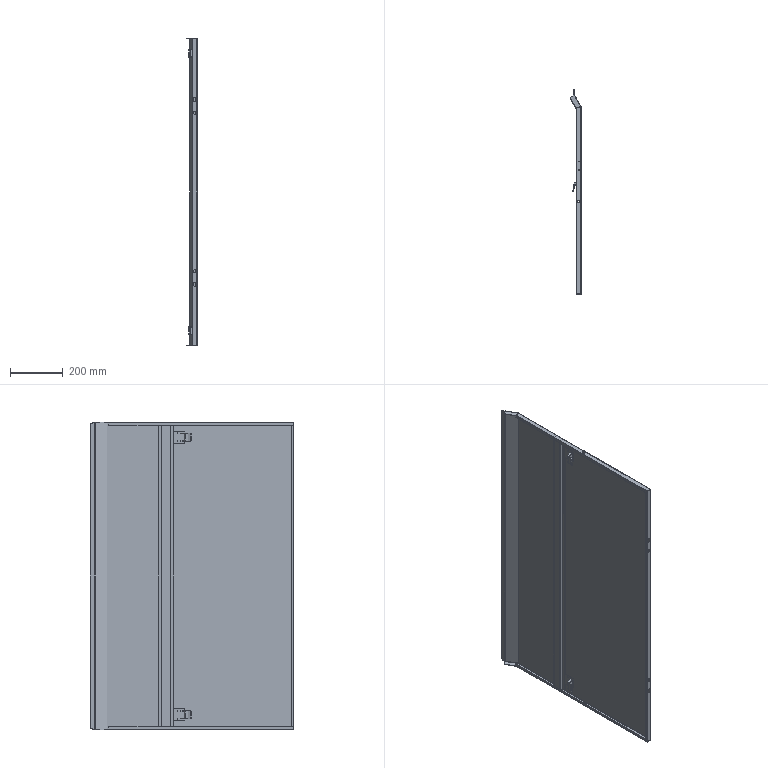Part | SolidWorks | features InContextFeatHolder 2 | 4 solids | 295 faces | box 40.015 x 773.5 x 1165 mm | volume 1625267 mm3 | plane 186 | cylinder 105 | spline 4 | commonest cylinder face diameters 0.4 x24 4 x18 3 x16 3.4 x14 4.4 x10 10 x8